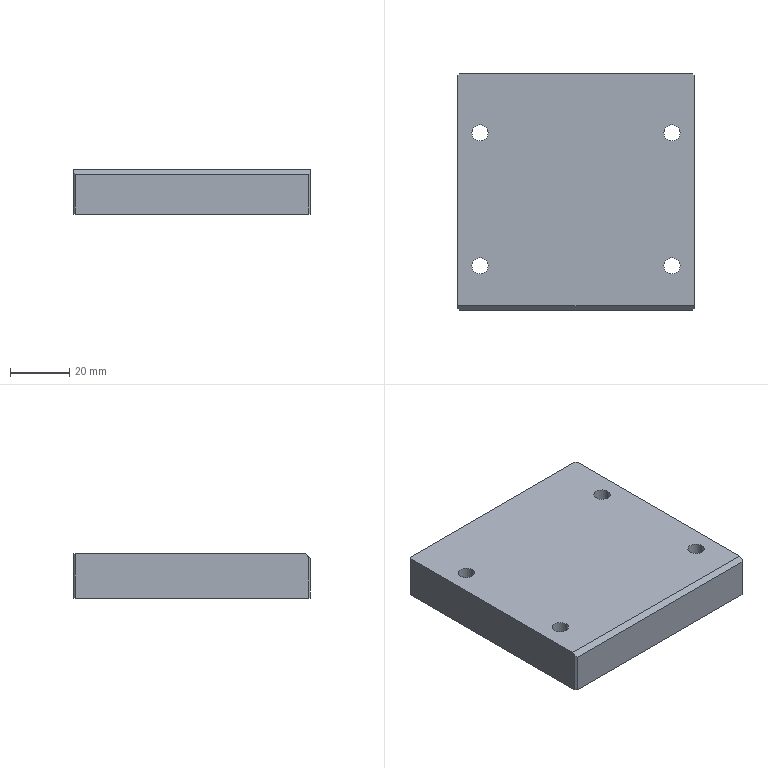Part | SolidWorks | features BaseBody 1 | 1 solid | 43 faces | box 80 x 80 x 15 mm | volume 92315 mm3 | cylinder 22 | plane 15 | cone 6 | commonest cylinder face diameters 5.5 x8 10 x8 5 x6
STEP:
#1=CARTESIAN_POINT('',(-27.5,-25.,5.7));
#2=VERTEX_POINT('',#1);
#3=CARTESIAN_POINT('',(-37.5,-25.,5.7));
#4=VERTEX_POINT('',#3);
#5=CARTESIAN_POINT('',(-32.5,-25.,5.7));
#6=DIRECTION('',(0.,0.,-1.));
#7=DIRECTION('',(-1.,0.,0.));
#8=AXIS2_PLACEMENT_3D('',#5,#6,#7);
#9=CIRCLE('',#8,5.);
#10=EDGE_CURVE('',#2,#4,#9,.T.);
#11=ORIENTED_EDGE('',*,*,#10,.F.);
#12=CARTESIAN_POINT('',(-27.5,-25.,0.));
#13=VERTEX_POINT('',#12);
#14=CARTESIAN_POINT('',(-27.5,-25.,0.));
#15=DIRECTION('',(0.,0.,-1.));
#16=VECTOR('',#15,1000.);
#17=LINE('',#14,#16);
#18=EDGE_CURVE('',#2,#13,#17,.T.);
#19=ORIENTED_EDGE('',*,*,#18,.T.);
#20=CARTESIAN_POINT('',(-37.5,-25.,0.));
#21=VERTEX_POINT('',#20);
#22=CARTESIAN_POINT('',(-32.5,-25.,0.));
#23=DIRECTION('',(0.,0.,-1.));
#24=DIRECTION('',(-1.,0.,0.));
#25=AXIS2_PLACEMENT_3D('',#22,#23,#24);
#26=CIRCLE('',#25,5.);
#27=EDGE_CURVE('',#13,#21,#26,.T.);
#28=ORIENTED_EDGE('',*,*,#27,.T.);
#29=CARTESIAN_POINT('',(-37.5,-25.,0.));
#30=DIRECTION('',(0.,0.,-1.));
#31=VECTOR('',#30,1000.);
#32=LINE('',#29,#31);
#33=EDGE_CURVE('',#4,#21,#32,.T.);
#34=ORIENTED_EDGE('',*,*,#33,.F.);
#35=EDGE_LOOP('',(#11,#19,#28,#34));
#36=FACE_OUTER_BOUND('',#35,.T.);
#37=CARTESIAN_POINT('',(-32.5,-25.,0.));
#38=DIRECTION('',(0.,0.,-1.));
#39=DIRECTION('',(-1.,0.,0.));
#40=AXIS2_PLACEMENT_3D('',#37,#38,#39);
#41=CYLINDRICAL_SURFACE('',#40,5.);
#42=ADVANCED_FACE('',(#36),#41,.F.);
#43=CARTESIAN_POINT('',(-29.75,-25.,15.));
#44=VERTEX_POINT('',#43);
#45=CARTESIAN_POINT('',(-35.25,-25.,15.));
#46=VERTEX_POINT('',#45);
#47=CARTESIAN_POINT('',(-32.5,-25.,15.));
#48=DIRECTION('',(0.,0.,-1.));
#49=DIRECTION('',(-1.,0.,0.));
#50=AXIS2_PLACEMENT_3D('',#47,#48,#49);
#51=CIRCLE('',#50,2.75);
#52=EDGE_CURVE('',#44,#46,#51,.T.);
#53=ORIENTED_EDGE('',*,*,#52,.F.);
#54=CARTESIAN_POINT('',(-29.75,-25.,5.7));
#55=VERTEX_POINT('',#54);
#56=CARTESIAN_POINT('',(-29.75,-25.,0.));
#57=DIRECTION('',(0.,0.,-1.));
#58=VECTOR('',#57,1000.);
#59=LINE('',#56,#58);
#60=EDGE_CURVE('',#44,#55,#59,.T.);
#61=ORIENTED_EDGE('',*,*,#60,.T.);
#62=CARTESIAN_POINT('',(-35.25,-25.,5.7));
#63=VERTEX_POINT('',#62);
#64=CARTESIAN_POINT('',(-32.5,-25.,5.7));
#65=DIRECTION('',(0.,0.,-1.));
#66=DIRECTION('',(-1.,0.,0.));
#67=AXIS2_PLACEMENT_3D('',#64,#65,#66);
#68=CIRCLE('',#67,2.75);
#69=EDGE_CURVE('',#55,#63,#68,.T.);
#70=ORIENTED_EDGE('',*,*,#69,.T.);
#71=CARTESIAN_POINT('',(-35.25,-25.,0.));
#72=DIRECTION('',(0.,0.,-1.));
#73=VECTOR('',#72,1000.);
#74=LINE('',#71,#73);
#75=EDGE_CURVE('',#46,#63,#74,.T.);
#76=ORIENTED_EDGE('',*,*,#75,.F.);
#77=EDGE_LOOP('',(#53,#61,#70,#76));
#78=FACE_OUTER_BOUND('',#77,.T.);
#79=CARTESIAN_POINT('',(-32.5,-25.,0.));
#80=DIRECTION('',(0.,0.,-1.));
#81=DIRECTION('',(-1.,0.,0.));
#82=AXIS2_PLACEMENT_3D('',#79,#80,#81);
#83=CYLINDRICAL_SURFACE('',#82,2.75);
#84=ADVANCED_FACE('',(#78),#83,.F.);
#85=CARTESIAN_POINT('',(-27.5,20.,5.7));
#86=VERTEX_POINT('',#85);
#87=CARTESIAN_POINT('',(-37.5,20.,5.7));
#88=VERTEX_POINT('',#87);
#89=CARTESIAN_POINT('',(-32.5,20.,5.7));
#90=DIRECTION('',(0.,0.,-1.));
#91=DIRECTION('',(-1.,0.,0.));
#92=AXIS2_PLACEMENT_3D('',#89,#90,#91);
#93=CIRCLE('',#92,5.);
#94=EDGE_CURVE('',#86,#88,#93,.T.);
#95=ORIENTED_EDGE('',*,*,#94,.F.);
#96=CARTESIAN_POINT('',(-27.5,20.,0.));
#97=VERTEX_POINT('',#96);
#98=CARTESIAN_POINT('',(-27.5,20.,0.));
#99=DIRECTION('',(0.,0.,-1.));
#100=VECTOR('',#99,1000.);
#101=LINE('',#98,#100);
#102=EDGE_CURVE('',#86,#97,#101,.T.);
#103=ORIENTED_EDGE('',*,*,#102,.T.);
#104=CARTESIAN_POINT('',(-37.5,20.,0.));
#105=VERTEX_POINT('',#104);
#106=CARTESIAN_POINT('',(-32.5,20.,0.));
#107=DIRECTION('',(0.,0.,-1.));
#108=DIRECTION('',(-1.,0.,0.));
#109=AXIS2_PLACEMENT_3D('',#106,#107,#108);
#110=CIRCLE('',#109,5.);
#111=EDGE_CURVE('',#97,#105,#110,.T.);
#112=ORIENTED_EDGE('',*,*,#111,.T.);
#113=CARTESIAN_POINT('',(-37.5,20.,0.));
#114=DIRECTION('',(0.,0.,-1.));
#115=VECTOR('',#114,1000.);
#116=LINE('',#113,#115);
#117=EDGE_CURVE('',#88,#105,#116,.T.);
#118=ORIENTED_EDGE('',*,*,#117,.F.);
#119=EDGE_LOOP('',(#95,#103,#112,#118));
#120=FACE_OUTER_BOUND('',#119,.T.);
#121=CARTESIAN_POINT('',(-32.5,20.,0.));
#122=DIRECTION('',(0.,0.,-1.));
#123=DIRECTION('',(-1.,0.,0.));
#124=AXIS2_PLACEMENT_3D('',#121,#122,#123);
#125=CYLINDRICAL_SURFACE('',#124,5.);
#126=ADVANCED_FACE('',(#120),#125,.F.);
#127=CARTESIAN_POINT('',(-29.75,20.,15.));
#128=VERTEX_POINT('',#127);
#129=CARTESIAN_POINT('',(-35.25,20.,15.));
#130=VERTEX_POINT('',#129);
#131=CARTESIAN_POINT('',(-32.5,20.,15.));
#132=DIRECTION('',(0.,0.,-1.));
#133=DIRECTION('',(-1.,0.,0.));
#134=AXIS2_PLACEMENT_3D('',#131,#132,#133);
#135=CIRCLE('',#134,2.75);
#136=EDGE_CURVE('',#128,#130,#135,.T.);
#137=ORIENTED_EDGE('',*,*,#136,.F.);
#138=CARTESIAN_POINT('',(-29.75,20.,5.7));
#139=VERTEX_POINT('',#138);
#140=CARTESIAN_POINT('',(-29.75,20.,0.));
#141=DIRECTION('',(0.,0.,-1.));
#142=VECTOR('',#141,1000.);
#143=LINE('',#140,#142);
#144=EDGE_CURVE('',#128,#139,#143,.T.);
#145=ORIENTED_EDGE('',*,*,#144,.T.);
#146=CARTESIAN_POINT('',(-35.25,20.,5.7));
#147=VERTEX_POINT('',#146);
#148=CARTESIAN_POINT('',(-32.5,20.,5.7));
#149=DIRECTION('',(0.,0.,-1.));
#150=DIRECTION('',(-1.,0.,0.));
#151=AXIS2_PLACEMENT_3D('',#148,#149,#150);
#152=CIRCLE('',#151,2.75);
#153=EDGE_CURVE('',#139,#147,#152,.T.);
#154=ORIENTED_EDGE('',*,*,#153,.T.);
#155=CARTESIAN_POINT('',(-35.25,20.,0.));
#156=DIRECTION('',(0.,0.,-1.));
#157=VECTOR('',#156,1000.);
#158=LINE('',#155,#157);
#159=EDGE_CURVE('',#130,#147,#158,.T.);
#160=ORIENTED_EDGE('',*,*,#159,.F.);
#161=EDGE_LOOP('',(#137,#145,#154,#160));
#162=FACE_OUTER_BOUND('',#161,.T.);
#163=CARTESIAN_POINT('',(-32.5,20.,0.));
#164=DIRECTION('',(0.,0.,-1.));
#165=DIRECTION('',(-1.,0.,0.));
#166=AXIS2_PLACEMENT_3D('',#163,#164,#165);
#167=CYLINDRICAL_SURFACE('',#166,2.75);
#168=ADVANCED_FACE('',(#162),#167,.F.);
#169=CARTESIAN_POINT('',(37.5,20.,5.7));
#170=VERTEX_POINT('',#169);
#171=CARTESIAN_POINT('',(27.5,20.,5.7));
#172=VERTEX_POINT('',#171);
#173=CARTESIAN_POINT('',(32.5,20.,5.7));
#174=DIRECTION('',(0.,0.,-1.));
#175=DIRECTION('',(-1.,0.,0.));
#176=AXIS2_PLACEMENT_3D('',#173,#174,#175);
#177=CIRCLE('',#176,5.);
#178=EDGE_CURVE('',#170,#172,#177,.T.);
#179=ORIENTED_EDGE('',*,*,#178,.F.);
#180=CARTESIAN_POINT('',(37.5,20.,0.));
#181=VERTEX_POINT('',#180);
#182=CARTESIAN_POINT('',(37.5,20.,0.));
#183=DIRECTION('',(0.,0.,-1.));
#184=VECTOR('',#183,1000.);
#185=LINE('',#182,#184);
#186=EDGE_CURVE('',#170,#181,#185,.T.);
#187=ORIENTED_EDGE('',*,*,#186,.T.);
#188=CARTESIAN_POINT('',(27.5,20.,0.));
#189=VERTEX_POINT('',#188);
#190=CARTESIAN_POINT('',(32.5,20.,0.));
#191=DIRECTION('',(0.,0.,-1.));
#192=DIRECTION('',(-1.,0.,0.));
#193=AXIS2_PLACEMENT_3D('',#190,#191,#192);
#194=CIRCLE('',#193,5.);
#195=EDGE_CURVE('',#181,#189,#194,.T.);
#196=ORIENTED_EDGE('',*,*,#195,.T.);
#197=CARTESIAN_POINT('',(27.5,20.,0.));
#198=DIRECTION('',(0.,0.,-1.));
#199=VECTOR('',#198,1000.);
#200=LINE('',#197,#199);
#201=EDGE_CURVE('',#172,#189,#200,.T.);
#202=ORIENTED_EDGE('',*,*,#201,.F.);
#203=EDGE_LOOP('',(#179,#187,#196,#202));
#204=FACE_OUTER_BOUND('',#203,.T.);
#205=CARTESIAN_POINT('',(32.5,20.,0.));
#206=DIRECTION('',(0.,0.,-1.));
#207=DIRECTION('',(-1.,0.,0.));
#208=AXIS2_PLACEMENT_3D('',#205,#206,#207);
#209=CYLINDRICAL_SURFACE('',#208,5.);
#210=ADVANCED_FACE('',(#204),#209,.F.);
#211=CARTESIAN_POINT('',(35.25,20.,15.));
#212=VERTEX_POINT('',#211);
#213=CARTESIAN_POINT('',(29.75,20.,15.));
#214=VERTEX_POINT('',#213);
#215=CARTESIAN_POINT('',(32.5,20.,15.));
#216=DIRECTION('',(0.,0.,-1.));
#217=DIRECTION('',(-1.,0.,0.));
#218=AXIS2_PLACEMENT_3D('',#215,#216,#217);
#219=CIRCLE('',#218,2.75);
#220=EDGE_CURVE('',#212,#214,#219,.T.);
#221=ORIENTED_EDGE('',*,*,#220,.F.);
#222=CARTESIAN_POINT('',(35.25,20.,5.7));
#223=VERTEX_POINT('',#222);
#224=CARTESIAN_POINT('',(35.25,20.,0.));
#225=DIRECTION('',(0.,0.,-1.));
#226=VECTOR('',#225,1000.);
#227=LINE('',#224,#226);
#228=EDGE_CURVE('',#212,#223,#227,.T.);
#229=ORIENTED_EDGE('',*,*,#228,.T.);
#230=CARTESIAN_POINT('',(29.75,20.,5.7));
#231=VERTEX_POINT('',#230);
#232=CARTESIAN_POINT('',(32.5,20.,5.7));
#233=DIRECTION('',(0.,0.,-1.));
#234=DIRECTION('',(-1.,0.,0.));
#235=AXIS2_PLACEMENT_3D('',#232,#233,#234);
#236=CIRCLE('',#235,2.75);
#237=EDGE_CURVE('',#223,#231,#236,.T.);
#238=ORIENTED_EDGE('',*,*,#237,.T.);
#239=CARTESIAN_POINT('',(29.75,20.,0.));
#240=DIRECTION('',(0.,0.,-1.));
#241=VECTOR('',#240,1000.);
#242=LINE('',#239,#241);
#243=EDGE_CURVE('',#214,#231,#242,.T.);
#244=ORIENTED_EDGE('',*,*,#243,.F.);
#245=EDGE_LOOP('',(#221,#229,#238,#244));
#246=FACE_OUTER_BOUND('',#245,.T.);
#247=CARTESIAN_POINT('',(32.5,20.,0.));
#248=DIRECTION('',(0.,0.,-1.));
#249=DIRECTION('',(-1.,0.,0.));
#250=AXIS2_PLACEMENT_3D('',#247,#248,#249);
#251=CYLINDRICAL_SURFACE('',#250,2.75);
#252=ADVANCED_FACE('',(#246),#251,.F.);
#253=CARTESIAN_POINT('',(37.5,-25.,5.7));
#254=VERTEX_POINT('',#253);
#255=CARTESIAN_POINT('',(27.5,-25.,5.7));
#256=VERTEX_POINT('',#255);
#257=CARTESIAN_POINT('',(32.5,-25.,5.7));
#258=DIRECTION('',(0.,0.,-1.));
#259=DIRECTION('',(-1.,0.,0.));
#260=AXIS2_PLACEMENT_3D('',#257,#258,#259);
#261=CIRCLE('',#260,5.);
#262=EDGE_CURVE('',#254,#256,#261,.T.);
#263=ORIENTED_EDGE('',*,*,#262,.F.);
#264=CARTESIAN_POINT('',(37.5,-25.,0.));
#265=VERTEX_POINT('',#264);
#266=CARTESIAN_POINT('',(37.5,-25.,0.));
#267=DIRECTION('',(0.,0.,-1.));
#268=VECTOR('',#267,1000.);
#269=LINE('',#266,#268);
#270=EDGE_CURVE('',#254,#265,#269,.T.);
#271=ORIENTED_EDGE('',*,*,#270,.T.);
#272=CARTESIAN_POINT('',(27.5,-25.,0.));
#273=VERTEX_POINT('',#272);
#274=CARTESIAN_POINT('',(32.5,-25.,0.));
#275=DIRECTION('',(0.,0.,-1.));
#276=DIRECTION('',(-1.,0.,0.));
#277=AXIS2_PLACEMENT_3D('',#274,#275,#276);
#278=CIRCLE('',#277,5.);
#279=EDGE_CURVE('',#265,#273,#278,.T.);
#280=ORIENTED_EDGE('',*,*,#279,.T.);
#281=CARTESIAN_POINT('',(27.5,-25.,0.));
#282=DIRECTION('',(0.,0.,-1.));
#283=VECTOR('',#282,1000.);
#284=LINE('',#281,#283);
#285=EDGE_CURVE('',#256,#273,#284,.T.);
#286=ORIENTED_EDGE('',*,*,#285,.F.);
#287=EDGE_LOOP('',(#263,#271,#280,#286));
#288=FACE_OUTER_BOUND('',#287,.T.);
#289=CARTESIAN_POINT('',(32.5,-25.,0.));
#290=DIRECTION('',(0.,0.,-1.));
#291=DIRECTION('',(-1.,0.,0.));
#292=AXIS2_PLACEMENT_3D('',#289,#290,#291);
#293=CYLINDRICAL_SURFACE('',#292,5.);
#294=ADVANCED_FACE('',(#288),#293,.F.);
#295=CARTESIAN_POINT('',(35.25,-25.,15.));
#296=VERTEX_POINT('',#295);
#297=CARTESIAN_POINT('',(29.75,-25.,15.));
#298=VERTEX_POINT('',#297);
#299=CARTESIAN_POINT('',(32.5,-25.,15.));
#300=DIRECTION('',(0.,0.,-1.));
#301=DIRECTION('',(-1.,0.,0.));
#302=AXIS2_PLACEMENT_3D('',#299,#300,#301);
#303=CIRCLE('',#302,2.75);
#304=EDGE_CURVE('',#296,#298,#303,.T.);
#305=ORIENTED_EDGE('',*,*,#304,.F.);
#306=CARTESIAN_POINT('',(35.25,-25.,5.7));
#307=VERTEX_POINT('',#306);
#308=CARTESIAN_POINT('',(35.25,-25.,0.));
#309=DIRECTION('',(0.,0.,-1.));
#310=VECTOR('',#309,1000.);
#311=LINE('',#308,#310);
#312=EDGE_CURVE('',#296,#307,#311,.T.);
#313=ORIENTED_EDGE('',*,*,#312,.T.);
#314=CARTESIAN_POINT('',(29.75,-25.,5.7));
#315=VERTEX_POINT('',#314);
#316=CARTESIAN_POINT('',(32.5,-25.,5.7));
#317=DIRECTION('',(0.,0.,-1.));
#318=DIRECTION('',(-1.,0.,0.));
#319=AXIS2_PLACEMENT_3D('',#316,#317,#318);
#320=CIRCLE('',#319,2.75);
#321=EDGE_CURVE('',#307,#315,#320,.T.);
#322=ORIENTED_EDGE('',*,*,#321,.T.);
#323=CARTESIAN_POINT('',(29.75,-25.,0.));
#324=DIRECTION('',(0.,0.,-1.));
#325=VECTOR('',#324,1000.);
#326=LINE('',#323,#325);
#327=EDGE_CURVE('',#298,#315,#326,.T.);
#328=ORIENTED_EDGE('',*,*,#327,.F.);
#329=EDGE_LOOP('',(#305,#313,#322,#328));
#330=FACE_OUTER_BOUND('',#329,.T.);
#331=CARTESIAN_POINT('',(32.5,-25.,0.));
#332=DIRECTION('',(0.,0.,-1.));
#333=DIRECTION('',(-1.,0.,0.));
#334=AXIS2_PLACEMENT_3D('',#331,#332,#333);
#335=CYLINDRICAL_SURFACE('',#334,2.75);
#336=ADVANCED_FACE('',(#330),#335,.F.);
#337=CARTESIAN_POINT('',(-27.5,25.,5.));
#338=VERTEX_POINT('',#337);
#339=CARTESIAN_POINT('',(-27.5,25.,10.));
#340=VERTEX_POINT('',#339);
#341=CARTESIAN_POINT('',(-27.5,25.,7.5));
#342=DIRECTION('',(0.,1.,0.));
#343=DIRECTION('',(0.,0.,1.));
#344=AXIS2_PLACEMENT_3D('',#341,#342,#343);
#345=CIRCLE('',#344,2.5);
#346=EDGE_CURVE('',#338,#340,#345,.T.);
#347=ORIENTED_EDGE('',*,*,#346,.F.);
#348=CARTESIAN_POINT('',(-27.5,40.,5.));
#349=VERTEX_POINT('',#348);
#350=CARTESIAN_POINT('',(-27.5,40.,5.));
#351=DIRECTION('',(0.,1.,0.));
#352=VECTOR('',#351,1000.);
#353=LINE('',#350,#352);
#354=EDGE_CURVE('',#338,#349,#353,.T.);
#355=ORIENTED_EDGE('',*,*,#354,.T.);
#356=CARTESIAN_POINT('',(-27.5,40.,10.));
#357=VERTEX_POINT('',#356);
#358=CARTESIAN_POINT('',(-27.5,40.,7.5));
#359=DIRECTION('',(0.,1.,0.));
#360=DIRECTION('',(0.,0.,1.));
#361=AXIS2_PLACEMENT_3D('',#358,#359,#360);
#362=CIRCLE('',#361,2.5);
#363=EDGE_CURVE('',#349,#357,#362,.T.);
#364=ORIENTED_EDGE('',*,*,#363,.T.);
#365=CARTESIAN_POINT('',(-27.5,40.,10.));
#366=DIRECTION('',(0.,1.,0.));
#367=VECTOR('',#366,1000.);
#368=LINE('',#365,#367);
#369=EDGE_CURVE('',#340,#357,#368,.T.);
#370=ORIENTED_EDGE('',*,*,#369,.F.);
#371=EDGE_LOOP('',(#347,#355,#364,#370));
#372=FACE_OUTER_BOUND('',#371,.T.);
#373=CARTESIAN_POINT('',(-27.5,40.,7.5));
#374=DIRECTION('',(0.,1.,0.));
#375=DIRECTION('',(0.,0.,1.));
#376=AXIS2_PLACEMENT_3D('',#373,#374,#375);
#377=CYLINDRICAL_SURFACE('',#376,2.5);
#378=ADVANCED_FACE('',(#372),#377,.F.);
#379=CARTESIAN_POINT('',(-27.5,23.498,7.5));
#380=VERTEX_POINT('',#379);
#381=CARTESIAN_POINT('',(-27.5,25.,10.));
#382=DIRECTION('',(0.,0.515,0.8572));
#383=VECTOR('',#382,1000.);
#384=LINE('',#381,#383);
#385=EDGE_CURVE('',#380,#340,#384,.T.);
#386=ORIENTED_EDGE('',*,*,#385,.F.);
#387=CARTESIAN_POINT('',(-27.5,25.,5.));
#388=DIRECTION('',(0.,0.515,-0.8572));
#389=VECTOR('',#388,1000.);
#390=LINE('',#387,#389);
#391=EDGE_CURVE('',#380,#338,#390,.T.);
#392=ORIENTED_EDGE('',*,*,#391,.T.);
#393=ORIENTED_EDGE('',*,*,#346,.T.);
#394=EDGE_LOOP('',(#386,#392,#393));
#395=FACE_OUTER_BOUND('',#394,.T.);
#396=CARTESIAN_POINT('',(-27.5,25.,7.5));
#397=DIRECTION('',(0.,1.,0.));
#398=DIRECTION('',(0.,0.,1.));
#399=AXIS2_PLACEMENT_3D('',#396,#397,#398);
#400=CONICAL_SURFACE('',#399,2.5,1.03);
#401=ADVANCED_FACE('',(#395),#400,.F.);
#402=CARTESIAN_POINT('',(0.,25.,5.));
#403=VERTEX_POINT('',#402);
#404=CARTESIAN_POINT('',(0.,25.,10.));
#405=VERTEX_POINT('',#404);
#406=CARTESIAN_POINT('',(0.,25.,7.5));
#407=DIRECTION('',(0.,1.,0.));
#408=DIRECTION('',(0.,0.,1.));
#409=AXIS2_PLACEMENT_3D('',#406,#407,#408);
#410=CIRCLE('',#409,2.5);
#411=EDGE_CURVE('',#403,#405,#410,.T.);
#412=ORIENTED_EDGE('',*,*,#411,.F.);
#413=CARTESIAN_POINT('',(0.,40.,5.));
#414=VERTEX_POINT('',#413);
#415=CARTESIAN_POINT('',(0.,40.,5.));
#416=DIRECTION('',(0.,1.,0.));
#417=VECTOR('',#416,1000.);
#418=LINE('',#415,#417);
#419=EDGE_CURVE('',#403,#414,#418,.T.);
#420=ORIENTED_EDGE('',*,*,#419,.T.);
#421=CARTESIAN_POINT('',(0.,40.,10.));
#422=VERTEX_POINT('',#421);
#423=CARTESIAN_POINT('',(0.,40.,7.5));
#424=DIRECTION('',(0.,1.,0.));
#425=DIRECTION('',(0.,0.,1.));
#426=AXIS2_PLACEMENT_3D('',#423,#424,#425);
#427=CIRCLE('',#426,2.5);
#428=EDGE_CURVE('',#414,#422,#427,.T.);
#429=ORIENTED_EDGE('',*,*,#428,.T.);
#430=CARTESIAN_POINT('',(0.,40.,10.));
#431=DIRECTION('',(0.,1.,0.));
#432=VECTOR('',#431,1000.);
#433=LINE('',#430,#432);
#434=EDGE_CURVE('',#405,#422,#433,.T.);
#435=ORIENTED_EDGE('',*,*,#434,.F.);
#436=EDGE_LOOP('',(#412,#420,#429,#435));
#437=FACE_OUTER_BOUND('',#436,.T.);
#438=CARTESIAN_POINT('',(0.,40.,7.5));
#439=DIRECTION('',(0.,1.,0.));
#440=DIRECTION('',(0.,0.,1.));
#441=AXIS2_PLACEMENT_3D('',#438,#439,#440);
#442=CYLINDRICAL_SURFACE('',#441,2.5);
#443=ADVANCED_FACE('',(#437),#442,.F.);
#444=CARTESIAN_POINT('',(0.,23.498,7.5));
#445=VERTEX_POINT('',#444);
#446=CARTESIAN_POINT('',(0.,25.,10.));
#447=DIRECTION('',(0.,0.515,0.8572));
#448=VECTOR('',#447,1000.);
#449=LINE('',#446,#448);
#450=EDGE_CURVE('',#445,#405,#449,.T.);
#451=ORIENTED_EDGE('',*,*,#450,.F.);
#452=CARTESIAN_POINT('',(0.,25.,5.));
#453=DIRECTION('',(0.,0.515,-0.8572));
#454=VECTOR('',#453,1000.);
#455=LINE('',#452,#454);
#456=EDGE_CURVE('',#445,#403,#455,.T.);
#457=ORIENTED_EDGE('',*,*,#456,.T.);
#458=ORIENTED_EDGE('',*,*,#411,.T.);
#459=EDGE_LOOP('',(#451,#457,#458));
#460=FACE_OUTER_BOUND('',#459,.T.);
#461=CARTESIAN_POINT('',(0.,25.,7.5));
#462=DIRECTION('',(0.,1.,0.));
#463=DIRECTION('',(0.,0.,1.));
#464=AXIS2_PLACEMENT_3D('',#461,#462,#463);
#465=CONICAL_SURFACE('',#464,2.5,1.03);
#466=ADVANCED_FACE('',(#460),#465,.F.);
#467=CARTESIAN_POINT('',(27.5,25.,5.));
#468=VERTEX_POINT('',#467);
#469=CARTESIAN_POINT('',(27.5,25.,10.));
#470=VERTEX_POINT('',#469);
#471=CARTESIAN_POINT('',(27.5,25.,7.5));
#472=DIRECTION('',(0.,1.,0.));
#473=DIRECTION('',(0.,0.,1.));
#474=AXIS2_PLACEMENT_3D('',#471,#472,#473);
#475=CIRCLE('',#474,2.5);
#476=EDGE_CURVE('',#468,#470,#475,.T.);
#477=ORIENTED_EDGE('',*,*,#476,.F.);
#478=CARTESIAN_POINT('',(27.5,40.,5.));
#479=VERTEX_POINT('',#478);
#480=CARTESIAN_POINT('',(27.5,40.,5.));
#481=DIRECTION('',(0.,1.,0.));
#482=VECTOR('',#481,1000.);
#483=LINE('',#480,#482);
#484=EDGE_CURVE('',#468,#479,#483,.T.);
#485=ORIENTED_EDGE('',*,*,#484,.T.);
#486=CARTESIAN_POINT('',(27.5,40.,10.));
#487=VERTEX_POINT('',#486);
#488=CARTESIAN_POINT('',(27.5,40.,7.5));
#489=DIRECTION('',(0.,1.,0.));
#490=DIRECTION('',(0.,0.,1.));
#491=AXIS2_PLACEMENT_3D('',#488,#489,#490);
#492=CIRCLE('',#491,2.5);
#493=EDGE_CURVE('',#479,#487,#492,.T.);
#494=ORIENTED_EDGE('',*,*,#493,.T.);
#495=CARTESIAN_POINT('',(27.5,40.,10.));
#496=DIRECTION('',(0.,1.,0.));
#497=VECTOR('',#496,1000.);
#498=LINE('',#495,#497);
#499=EDGE_CURVE('',#470,#487,#498,.T.);
#500=ORIENTED_EDGE('',*,*,#499,.F.);
#501=EDGE_LOOP('',(#477,#485,#494,#500));
#502=FACE_OUTER_BOUND('',#501,.T.);
#503=CARTESIAN_POINT('',(27.5,40.,7.5));
#504=DIRECTION('',(0.,1.,0.));
#505=DIRECTION('',(0.,0.,1.));
#506=AXIS2_PLACEMENT_3D('',#503,#504,#505);
#507=CYLINDRICAL_SURFACE('',#506,2.5);
#508=ADVANCED_FACE('',(#502),#507,.F.);
#509=CARTESIAN_POINT('',(27.5,23.498,7.5));
#510=VERTEX_POINT('',#509);
#511=CARTESIAN_POINT('',(27.5,25.,10.));
#512=DIRECTION('',(0.,0.515,0.8572));
#513=VECTOR('',#512,1000.);
#514=LINE('',#511,#513);
#515=EDGE_CURVE('',#510,#470,#514,.T.);
#516=ORIENTED_EDGE('',*,*,#515,.F.);
#517=CARTESIAN_POINT('',(27.5,25.,5.));
#518=DIRECTION('',(0.,0.515,-0.8572));
#519=VECTOR('',#518,1000.);
#520=LINE('',#517,#519);
#521=EDGE_CURVE('',#510,#468,#520,.T.);
#522=ORIENTED_EDGE('',*,*,#521,.T.);
#523=ORIENTED_EDGE('',*,*,#476,.T.);
#524=EDGE_LOOP('',(#516,#522,#523));
#525=FACE_OUTER_BOUND('',#524,.T.);
#526=CARTESIAN_POINT('',(27.5,25.,7.5));
#527=DIRECTION('',(0.,1.,0.));
#528=DIRECTION('',(0.,0.,1.));
#529=AXIS2_PLACEMENT_3D('',#526,#527,#528);
#530=CONICAL_SURFACE('',#529,2.5,1.03);
#531=ADVANCED_FACE('',(#525),#530,.F.);
#532=CARTESIAN_POINT('',(-39.5,-40.,13.5));
#533=VERTEX_POINT('',#532);
#534=CARTESIAN_POINT('',(-40.,-39.5,14.));
#535=VERTEX_POINT('',#534);
#536=CARTESIAN_POINT('',(-40.,-39.5,14.));
#537=DIRECTION('',(-0.5774,0.5774,0.5774));
#538=VECTOR('',#537,1000.);
#539=LINE('',#536,#538);
#540=EDGE_CURVE('',#533,#535,#539,.T.);
#541=ORIENTED_EDGE('',*,*,#540,.F.);
#542=CARTESIAN_POINT('',(39.5,-40.,13.5));
#543=VERTEX_POINT('',#542);
#544=CARTESIAN_POINT('',(-40.,-40.,13.5));
#545=DIRECTION('',(-1.,0.,0.));
#546=VECTOR('',#545,1000.);
#547=LINE('',#544,#546);
#548=EDGE_CURVE('',#543,#533,#547,.T.);
#549=ORIENTED_EDGE('',*,*,#548,.F.);
#550=CARTESIAN_POINT('',(40.,-39.5,14.));
#551=VERTEX_POINT('',#550);
#552=CARTESIAN_POINT('',(40.333,-39.167,14.333));
#553=DIRECTION('',(-0.5774,-0.5774,-0.5774));
#554=VECTOR('',#553,1000.);
#555=LINE('',#552,#554);
#556=EDGE_CURVE('',#551,#543,#555,.T.);
#557=ORIENTED_EDGE('',*,*,#556,.F.);
#558=CARTESIAN_POINT('',(40.,-38.5,15.));
#559=VERTEX_POINT('',#558);
#560=CARTESIAN_POINT('',(40.,-38.5,15.));
#561=DIRECTION('',(0.,-0.7071,-0.7071));
#562=VECTOR('',#561,1000.);
#563=LINE('',#560,#562);
#564=EDGE_CURVE('',#559,#551,#563,.T.);
#565=ORIENTED_EDGE('',*,*,#564,.F.);
#566=CARTESIAN_POINT('',(-40.,-38.5,15.));
#567=VERTEX_POINT('',#566);
#568=CARTESIAN_POINT('',(0.,-38.5,15.));
#569=DIRECTION('',(1.,0.,0.));
#570=VECTOR('',#569,1000.);
#571=LINE('',#568,#570);
#572=EDGE_CURVE('',#567,#559,#571,.T.);
#573=ORIENTED_EDGE('',*,*,#572,.F.);
#574=CARTESIAN_POINT('',(-40.,-38.5,15.));
#575=DIRECTION('',(0.,0.7071,0.7071));
#576=VECTOR('',#575,1000.);
#577=LINE('',#574,#576);
#578=EDGE_CURVE('',#535,#567,#577,.T.);
#579=ORIENTED_EDGE('',*,*,#578,.F.);
#580=EDGE_LOOP('',(#541,#549,#557,#565,#573,#579));
#581=FACE_OUTER_BOUND('',#580,.T.);
#582=CARTESIAN_POINT('',(0.,-38.5,15.));
#583=DIRECTION('',(0.,0.7071,-0.7071));
#584=DIRECTION('',(-1.,0.,0.));
#585=AXIS2_PLACEMENT_3D('',#582,#583,#584);
#586=PLANE('',#585);
#587=ADVANCED_FACE('',(#581),#586,.F.);
#588=CARTESIAN_POINT('',(40.,-39.5,0.));
#589=VERTEX_POINT('',#588);
#590=CARTESIAN_POINT('',(40.,-39.5,15.));
#591=DIRECTION('',(0.,0.,-1.));
#592=VECTOR('',#591,1000.);
#593=LINE('',#590,#592);
#594=EDGE_CURVE('',#551,#589,#593,.T.);
#595=ORIENTED_EDGE('',*,*,#594,.F.);
#596=ORIENTED_EDGE('',*,*,#556,.T.);
#597=CARTESIAN_POINT('',(39.5,-40.,0.));
#598=VERTEX_POINT('',#597);
#599=CARTESIAN_POINT('',(39.5,-40.,15.));
#600=DIRECTION('',(0.,0.,1.));
#601=VECTOR('',#600,1000.);
#602=LINE('',#599,#601);
#603=EDGE_CURVE('',#598,#543,#602,.T.);
#604=ORIENTED_EDGE('',*,*,#603,.F.);
#605=CARTESIAN_POINT('',(39.75,-39.75,0.));
#606=DIRECTION('',(-0.7071,-0.7071,0.));
#607=VECTOR('',#606,1000.);
#608=LINE('',#605,#607);
#609=EDGE_CURVE('',#589,#598,#608,.T.);
#610=ORIENTED_EDGE('',*,*,#609,.F.);
#611=EDGE_LOOP('',(#595,#596,#604,#610));
#612=FACE_OUTER_BOUND('',#611,.T.);
#613=CARTESIAN_POINT('',(40.,-39.5,15.));
#614=DIRECTION('',(-0.7071,0.7071,0.));
#615=DIRECTION('',(0.,0.,1.));
#616=AXIS2_PLACEMENT_3D('',#613,#614,#615);
#617=PLANE('',#616);
#618=ADVANCED_FACE('',(#612),#617,.F.);
#619=CARTESIAN_POINT('',(-39.5,-40.,0.));
#620=VERTEX_POINT('',#619);
#621=CARTESIAN_POINT('',(-39.5,-40.,15.));
#622=DIRECTION('',(0.,0.,-1.));
#623=VECTOR('',#622,1000.);
#624=LINE('',#621,#623);
#625=EDGE_CURVE('',#533,#620,#624,.T.);
#626=ORIENTED_EDGE('',*,*,#625,.F.);
#627=ORIENTED_EDGE('',*,*,#540,.T.);
#628=CARTESIAN_POINT('',(-40.,-39.5,0.));
#629=VERTEX_POINT('',#628);
#630=CARTESIAN_POINT('',(-40.,-39.5,15.));
#631=DIRECTION('',(0.,0.,1.));
#632=VECTOR('',#631,1000.);
#633=LINE('',#630,#632);
#634=EDGE_CURVE('',#629,#535,#633,.T.);
#635=ORIENTED_EDGE('',*,*,#634,.F.);
#636=CARTESIAN_POINT('',(-39.75,-39.75,0.));
#637=DIRECTION('',(-0.7071,0.7071,0.));
#638=VECTOR('',#637,1000.);
#639=LINE('',#636,#638);
#640=EDGE_CURVE('',#620,#629,#639,.T.);
#641=ORIENTED_EDGE('',*,*,#640,.F.);
#642=EDGE_LOOP('',(#626,#627,#635,#641));
#643=FACE_OUTER_BOUND('',#642,.T.);
#644=CARTESIAN_POINT('',(-39.5,-40.,15.));
#645=DIRECTION('',(0.7071,0.7071,0.));
#646=DIRECTION('',(0.,0.,-1.));
#647=AXIS2_PLACEMENT_3D('',#644,#645,#646);
#648=PLANE('',#647);
#649=ADVANCED_FACE('',(#643),#648,.F.);
#650=CARTESIAN_POINT('',(40.,39.5,15.));
#651=VERTEX_POINT('',#650);
#652=CARTESIAN_POINT('',(39.5,40.,15.));
#653=VERTEX_POINT('',#652);
#654=CARTESIAN_POINT('',(39.5,40.,15.));
#655=DIRECTION('',(-0.7071,0.7071,0.));
#656=VECTOR('',#655,1000.);
#657=LINE('',#654,#656);
#658=EDGE_CURVE('',#651,#653,#657,.T.);
#659=ORIENTED_EDGE('',*,*,#658,.F.);
#660=CARTESIAN_POINT('',(40.,39.5,0.));
#661=VERTEX_POINT('',#660);
#662=CARTESIAN_POINT('',(40.,39.5,15.));
#663=DIRECTION('',(0.,0.,1.));
#664=VECTOR('',#663,1000.);
#665=LINE('',#662,#664);
#666=EDGE_CURVE('',#661,#651,#665,.T.);
#667=ORIENTED_EDGE('',*,*,#666,.F.);
#668=CARTESIAN_POINT('',(39.5,40.,0.));
#669=VERTEX_POINT('',#668);
#670=CARTESIAN_POINT('',(39.75,39.75,0.));
#671=DIRECTION('',(0.7071,-0.7071,0.));
#672=VECTOR('',#671,1000.);
#673=LINE('',#670,#672);
#674=EDGE_CURVE('',#669,#661,#673,.T.);
#675=ORIENTED_EDGE('',*,*,#674,.F.);
#676=CARTESIAN_POINT('',(39.5,40.,15.));
#677=DIRECTION('',(0.,0.,-1.));
#678=VECTOR('',#677,1000.);
#679=LINE('',#676,#678);
#680=EDGE_CURVE('',#653,#669,#679,.T.);
#681=ORIENTED_EDGE('',*,*,#680,.F.);
#682=EDGE_LOOP('',(#659,#667,#675,#681));
#683=FACE_OUTER_BOUND('',#682,.T.);
#684=CARTESIAN_POINT('',(39.5,40.,15.));
#685=DIRECTION('',(-0.7071,-0.7071,0.));
#686=DIRECTION('',(-0.7071,0.7071,0.));
#687=AXIS2_PLACEMENT_3D('',#684,#685,#686);
#688=PLANE('',#687);
#689=ADVANCED_FACE('',(#683),#688,.F.);
#690=CARTESIAN_POINT('',(-39.5,40.,15.));
#691=VERTEX_POINT('',#690);
#692=CARTESIAN_POINT('',(-40.,39.5,15.));
#693=VERTEX_POINT('',#692);
#694=CARTESIAN_POINT('',(-40.,39.5,15.));
#695=DIRECTION('',(-0.7071,-0.7071,0.));
#696=VECTOR('',#695,1000.);
#697=LINE('',#694,#696);
#698=EDGE_CURVE('',#691,#693,#697,.T.);
#699=ORIENTED_EDGE('',*,*,#698,.F.);
#700=CARTESIAN_POINT('',(-39.5,40.,0.));
#701=VERTEX_POINT('',#700);
#702=CARTESIAN_POINT('',(-39.5,40.,15.));
#703=DIRECTION('',(0.,0.,1.));
#704=VECTOR('',#703,1000.);
#705=LINE('',#702,#704);
#706=EDGE_CURVE('',#701,#691,#705,.T.);
#707=ORIENTED_EDGE('',*,*,#706,.F.);
#708=CARTESIAN_POINT('',(-40.,39.5,0.));
#709=VERTEX_POINT('',#708);
#710=CARTESIAN_POINT('',(-39.75,39.75,0.));
#711=DIRECTION('',(0.7071,0.7071,0.));
#712=VECTOR('',#711,1000.);
#713=LINE('',#710,#712);
#714=EDGE_CURVE('',#709,#701,#713,.T.);
#715=ORIENTED_EDGE('',*,*,#714,.F.);
#716=CARTESIAN_POINT('',(-40.,39.5,15.));
#717=DIRECTION('',(0.,0.,-1.));
#718=VECTOR('',#717,1000.);
#719=LINE('',#716,#718);
#720=EDGE_CURVE('',#693,#709,#719,.T.);
#721=ORIENTED_EDGE('',*,*,#720,.F.);
#722=EDGE_LOOP('',(#699,#707,#715,#721));
#723=FACE_OUTER_BOUND('',#722,.T.);
#724=CARTESIAN_POINT('',(-40.,39.5,15.));
#725=DIRECTION('',(0.7071,-0.7071,0.));
#726=DIRECTION('',(0.,0.,-1.));
#727=AXIS2_PLACEMENT_3D('',#724,#725,#726);
#728=PLANE('',#727);
#729=ADVANCED_FACE('',(#723),#728,.F.);
#730=CARTESIAN_POINT('',(-32.5,-25.,5.7));
#731=DIRECTION('',(0.,0.,-1.));
#732=DIRECTION('',(-1.,0.,0.));
#733=AXIS2_PLACEMENT_3D('',#730,#731,#732);
#734=CIRCLE('',#733,2.75);
#735=EDGE_CURVE('',#63,#55,#734,.T.);
#736=ORIENTED_EDGE('',*,*,#735,.F.);
#737=ORIENTED_EDGE('',*,*,#69,.F.);
#738=EDGE_LOOP('',(#736,#737));
#739=FACE_BOUND('',#738,.T.);
#740=CARTESIAN_POINT('',(-32.5,-25.,5.7));
#741=DIRECTION('',(0.,0.,-1.));
#742=DIRECTION('',(-1.,0.,0.));
#743=AXIS2_PLACEMENT_3D('',#740,#741,#742);
#744=CIRCLE('',#743,5.);
#745=EDGE_CURVE('',#4,#2,#744,.T.);
#746=ORIENTED_EDGE('',*,*,#745,.T.);
#747=ORIENTED_EDGE('',*,*,#10,.T.);
#748=EDGE_LOOP('',(#746,#747));
#749=FACE_OUTER_BOUND('',#748,.T.);
#750=CARTESIAN_POINT('',(-29.75,-25.,5.7));
#751=DIRECTION('',(0.,0.,1.));
#752=DIRECTION('',(1.,0.,0.));
#753=AXIS2_PLACEMENT_3D('',#750,#751,#752);
#754=PLANE('',#753);
#755=ADVANCED_FACE('',(#739,#749),#754,.F.);
#756=CARTESIAN_POINT('',(-32.5,20.,5.7));
#757=DIRECTION('',(0.,0.,-1.));
#758=DIRECTION('',(-1.,0.,0.));
#759=AXIS2_PLACEMENT_3D('',#756,#757,#758);
#760=CIRCLE('',#759,2.75);
#761=EDGE_CURVE('',#147,#139,#760,.T.);
#762=ORIENTED_EDGE('',*,*,#761,.F.);
#763=ORIENTED_EDGE('',*,*,#153,.F.);
#764=EDGE_LOOP('',(#762,#763));
#765=FACE_BOUND('',#764,.T.);
#766=CARTESIAN_POINT('',(-32.5,20.,5.7));
#767=DIRECTION('',(0.,0.,-1.));
#768=DIRECTION('',(-1.,0.,0.));
#769=AXIS2_PLACEMENT_3D('',#766,#767,#768);
#770=CIRCLE('',#769,5.);
#771=EDGE_CURVE('',#88,#86,#770,.T.);
#772=ORIENTED_EDGE('',*,*,#771,.T.);
#773=ORIENTED_EDGE('',*,*,#94,.T.);
#774=EDGE_LOOP('',(#772,#773));
#775=FACE_OUTER_BOUND('',#774,.T.);
#776=CARTESIAN_POINT('',(-29.75,20.,5.7));
#777=DIRECTION('',(0.,0.,1.));
#778=DIRECTION('',(1.,0.,0.));
#779=AXIS2_PLACEMENT_3D('',#776,#777,#778);
#780=PLANE('',#779);
#781=ADVANCED_FACE('',(#765,#775),#780,.F.);
#782=CARTESIAN_POINT('',(32.5,20.,5.7));
#783=DIRECTION('',(0.,0.,-1.));
#784=DIRECTION('',(-1.,0.,0.));
#785=AXIS2_PLACEMENT_3D('',#782,#783,#784);
#786=CIRCLE('',#785,2.75);
#787=EDGE_CURVE('',#231,#223,#786,.T.);
#788=ORIENTED_EDGE('',*,*,#787,.F.);
#789=ORIENTED_EDGE('',*,*,#237,.F.);
#790=EDGE_LOOP('',(#788,#789));
#791=FACE_BOUND('',#790,.T.);
#792=CARTESIAN_POINT('',(32.5,20.,5.7));
#793=DIRECTION('',(0.,0.,-1.));
#794=DIRECTION('',(-1.,0.,0.));
#795=AXIS2_PLACEMENT_3D('',#792,#793,#794);
#796=CIRCLE('',#795,5.);
#797=EDGE_CURVE('',#172,#170,#796,.T.);
#798=ORIENTED_EDGE('',*,*,#797,.T.);
#799=ORIENTED_EDGE('',*,*,#178,.T.);
#800=EDGE_LOOP('',(#798,#799));
#801=FACE_OUTER_BOUND('',#800,.T.);
#802=CARTESIAN_POINT('',(35.25,20.,5.7));
#803=DIRECTION('',(0.,0.,1.));
#804=DIRECTION('',(1.,0.,0.));
#805=AXIS2_PLACEMENT_3D('',#802,#803,#804);
#806=PLANE('',#805);
#807=ADVANCED_FACE('',(#791,#801),#806,.F.);
#808=CARTESIAN_POINT('',(32.5,-25.,5.7));
#809=DIRECTION('',(0.,0.,-1.));
#810=DIRECTION('',(-1.,0.,0.));
#811=AXIS2_PLACEMENT_3D('',#808,#809,#810);
#812=CIRCLE('',#811,2.75);
#813=EDGE_CURVE('',#315,#307,#812,.T.);
#814=ORIENTED_EDGE('',*,*,#813,.F.);
#815=ORIENTED_EDGE('',*,*,#321,.F.);
#816=EDGE_LOOP('',(#814,#815));
#817=FACE_BOUND('',#816,.T.);
#818=CARTESIAN_POINT('',(32.5,-25.,5.7));
#819=DIRECTION('',(0.,0.,-1.));
#820=DIRECTION('',(-1.,0.,0.));
#821=AXIS2_PLACEMENT_3D('',#818,#819,#820);
#822=CIRCLE('',#821,5.);
#823=EDGE_CURVE('',#256,#254,#822,.T.);
#824=ORIENTED_EDGE('',*,*,#823,.T.);
#825=ORIENTED_EDGE('',*,*,#262,.T.);
#826=EDGE_LOOP('',(#824,#825));
#827=FACE_OUTER_BOUND('',#826,.T.);
#828=CARTESIAN_POINT('',(35.25,-25.,5.7));
#829=DIRECTION('',(0.,0.,1.));
#830=DIRECTION('',(1.,0.,0.));
#831=AXIS2_PLACEMENT_3D('',#828,#829,#830);
#832=PLANE('',#831);
#833=ADVANCED_FACE('',(#817,#827),#832,.F.);
#834=CARTESIAN_POINT('',(32.5,-25.,0.));
#835=DIRECTION('',(0.,0.,-1.));
#836=DIRECTION('',(-1.,0.,0.));
#837=AXIS2_PLACEMENT_3D('',#834,#835,#836);
#838=CIRCLE('',#837,5.);
#839=EDGE_CURVE('',#273,#265,#838,.T.);
#840=ORIENTED_EDGE('',*,*,#839,.F.);
#841=ORIENTED_EDGE('',*,*,#279,.F.);
#842=EDGE_LOOP('',(#840,#841));
#843=FACE_BOUND('',#842,.T.);
#844=CARTESIAN_POINT('',(32.5,20.,0.));
#845=DIRECTION('',(0.,0.,-1.));
#846=DIRECTION('',(-1.,0.,0.));
#847=AXIS2_PLACEMENT_3D('',#844,#845,#846);
#848=CIRCLE('',#847,5.);
#849=EDGE_CURVE('',#189,#181,#848,.T.);
#850=ORIENTED_EDGE('',*,*,#849,.F.);
#851=ORIENTED_EDGE('',*,*,#195,.F.);
#852=EDGE_LOOP('',(#850,#851));
#853=FACE_BOUND('',#852,.T.);
#854=CARTESIAN_POINT('',(-32.5,20.,0.));
#855=DIRECTION('',(0.,0.,-1.));
#856=DIRECTION('',(-1.,0.,0.));
#857=AXIS2_PLACEMENT_3D('',#854,#855,#856);
#858=CIRCLE('',#857,5.);
#859=EDGE_CURVE('',#105,#97,#858,.T.);
#860=ORIENTED_EDGE('',*,*,#859,.F.);
#861=ORIENTED_EDGE('',*,*,#111,.F.);
#862=EDGE_LOOP('',(#860,#861));
#863=FACE_BOUND('',#862,.T.);
#864=CARTESIAN_POINT('',(-32.5,-25.,0.));
#865=DIRECTION('',(0.,0.,-1.));
#866=DIRECTION('',(-1.,0.,0.));
#867=AXIS2_PLACEMENT_3D('',#864,#865,#866);
#868=CIRCLE('',#867,5.);
#869=EDGE_CURVE('',#21,#13,#868,.T.);
#870=ORIENTED_EDGE('',*,*,#869,.F.);
#871=ORIENTED_EDGE('',*,*,#27,.F.);
#872=EDGE_LOOP('',(#870,#871));
#873=FACE_BOUND('',#872,.T.);
#874=CARTESIAN_POINT('',(-40.,-40.,0.));
#875=DIRECTION('',(0.,-1.,0.));
#876=VECTOR('',#875,1000.);
#877=LINE('',#874,#876);
#878=EDGE_CURVE('',#709,#629,#877,.T.);
#879=ORIENTED_EDGE('',*,*,#878,.F.);
#880=ORIENTED_EDGE('',*,*,#714,.T.);
#881=CARTESIAN_POINT('',(-40.,40.,0.));
#882=DIRECTION('',(-1.,0.,0.));
#883=VECTOR('',#882,1000.);
#884=LINE('',#881,#883);
#885=EDGE_CURVE('',#669,#701,#884,.T.);
#886=ORIENTED_EDGE('',*,*,#885,.F.);
#887=ORIENTED_EDGE('',*,*,#674,.T.);
#888=CARTESIAN_POINT('',(40.,-40.,0.));
#889=DIRECTION('',(0.,1.,0.));
#890=VECTOR('',#889,1000.);
#891=LINE('',#888,#890);
#892=EDGE_CURVE('',#589,#661,#891,.T.);
#893=ORIENTED_EDGE('',*,*,#892,.F.);
#894=ORIENTED_EDGE('',*,*,#609,.T.);
#895=CARTESIAN_POINT('',(-40.,-40.,0.));
#896=DIRECTION('',(1.,0.,0.));
#897=VECTOR('',#896,1000.);
#898=LINE('',#895,#897);
#899=EDGE_CURVE('',#620,#598,#898,.T.);
#900=ORIENTED_EDGE('',*,*,#899,.F.);
#901=ORIENTED_EDGE('',*,*,#640,.T.);
#902=EDGE_LOOP('',(#879,#880,#886,#887,#893,#894,#900,#901));
#903=FACE_OUTER_BOUND('',#902,.T.);
#904=CARTESIAN_POINT('',(0.,0.,0.));
#905=DIRECTION('',(0.,0.,-1.));
#906=DIRECTION('',(0.,-1.,0.));
#907=AXIS2_PLACEMENT_3D('',#904,#905,#906);
#908=PLANE('',#907);
#909=ADVANCED_FACE('',(#843,#853,#863,#873,#903),#908,.T.);
#910=CARTESIAN_POINT('',(32.5,-25.,15.));
#911=DIRECTION('',(0.,0.,-1.));
#912=DIRECTION('',(-1.,0.,0.));
#913=AXIS2_PLACEMENT_3D('',#910,#911,#912);
#914=CIRCLE('',#913,2.75);
#915=EDGE_CURVE('',#298,#296,#914,.T.);
#916=ORIENTED_EDGE('',*,*,#915,.T.);
#917=ORIENTED_EDGE('',*,*,#304,.T.);
#918=EDGE_LOOP('',(#916,#917));
#919=FACE_BOUND('',#918,.T.);
#920=CARTESIAN_POINT('',(32.5,20.,15.));
#921=DIRECTION('',(0.,0.,-1.));
#922=DIRECTION('',(-1.,0.,0.));
#923=AXIS2_PLACEMENT_3D('',#920,#921,#922);
#924=CIRCLE('',#923,2.75);
#925=EDGE_CURVE('',#214,#212,#924,.T.);
#926=ORIENTED_EDGE('',*,*,#925,.T.);
#927=ORIENTED_EDGE('',*,*,#220,.T.);
#928=EDGE_LOOP('',(#926,#927));
#929=FACE_BOUND('',#928,.T.);
#930=CARTESIAN_POINT('',(-32.5,20.,15.));
#931=DIRECTION('',(0.,0.,-1.));
#932=DIRECTION('',(-1.,0.,0.));
#933=AXIS2_PLACEMENT_3D('',#930,#931,#932);
#934=CIRCLE('',#933,2.75);
#935=EDGE_CURVE('',#130,#128,#934,.T.);
#936=ORIENTED_EDGE('',*,*,#935,.T.);
#937=ORIENTED_EDGE('',*,*,#136,.T.);
#938=EDGE_LOOP('',(#936,#937));
#939=FACE_BOUND('',#938,.T.);
#940=CARTESIAN_POINT('',(-32.5,-25.,15.));
#941=DIRECTION('',(0.,0.,-1.));
#942=DIRECTION('',(-1.,0.,0.));
#943=AXIS2_PLACEMENT_3D('',#940,#941,#942);
#944=CIRCLE('',#943,2.75);
#945=EDGE_CURVE('',#46,#44,#944,.T.);
#946=ORIENTED_EDGE('',*,*,#945,.T.);
#947=ORIENTED_EDGE('',*,*,#52,.T.);
#948=EDGE_LOOP('',(#946,#947));
#949=FACE_BOUND('',#948,.T.);
#950=CARTESIAN_POINT('',(-40.,-40.,15.));
#951=DIRECTION('',(0.,-1.,0.));
#952=VECTOR('',#951,1000.);
#953=LINE('',#950,#952);
#954=EDGE_CURVE('',#693,#567,#953,.T.);
#955=ORIENTED_EDGE('',*,*,#954,.T.);
#956=ORIENTED_EDGE('',*,*,#572,.T.);
#957=CARTESIAN_POINT('',(40.,-40.,15.));
#958=DIRECTION('',(0.,1.,0.));
#959=VECTOR('',#958,1000.);
#960=LINE('',#957,#959);
#961=EDGE_CURVE('',#559,#651,#960,.T.);
#962=ORIENTED_EDGE('',*,*,#961,.T.);
#963=ORIENTED_EDGE('',*,*,#658,.T.);
#964=CARTESIAN_POINT('',(-40.,40.,15.));
#965=DIRECTION('',(-1.,0.,0.));
#966=VECTOR('',#965,1000.);
#967=LINE('',#964,#966);
#968=EDGE_CURVE('',#653,#691,#967,.T.);
#969=ORIENTED_EDGE('',*,*,#968,.T.);
#970=ORIENTED_EDGE('',*,*,#698,.T.);
#971=EDGE_LOOP('',(#955,#956,#962,#963,#969,#970));
#972=FACE_OUTER_BOUND('',#971,.T.);
#973=CARTESIAN_POINT('',(0.,0.,15.));
#974=DIRECTION('',(0.,0.,-1.));
#975=DIRECTION('',(0.,-1.,0.));
#976=AXIS2_PLACEMENT_3D('',#973,#974,#975);
#977=PLANE('',#976);
#978=ADVANCED_FACE('',(#919,#929,#939,#949,#972),#977,.F.);
#979=CARTESIAN_POINT('',(27.5,40.,7.5));
#980=DIRECTION('',(0.,1.,0.));
#981=DIRECTION('',(0.,0.,1.));
#982=AXIS2_PLACEMENT_3D('',#979,#980,#981);
#983=CIRCLE('',#982,2.5);
#984=EDGE_CURVE('',#487,#479,#983,.T.);
#985=ORIENTED_EDGE('',*,*,#984,.F.);
#986=ORIENTED_EDGE('',*,*,#493,.F.);
#987=EDGE_LOOP('',(#985,#986));
#988=FACE_BOUND('',#987,.T.);
#989=CARTESIAN_POINT('',(0.,40.,7.5));
#990=DIRECTION('',(0.,1.,0.));
#991=DIRECTION('',(0.,0.,1.));
#992=AXIS2_PLACEMENT_3D('',#989,#990,#991);
#993=CIRCLE('',#992,2.5);
#994=EDGE_CURVE('',#422,#414,#993,.T.);
#995=ORIENTED_EDGE('',*,*,#994,.F.);
#996=ORIENTED_EDGE('',*,*,#428,.F.);
#997=EDGE_LOOP('',(#995,#996));
#998=FACE_BOUND('',#997,.T.);
#999=CARTESIAN_POINT('',(-27.5,40.,7.5));
#1000=DIRECTION('',(0.,1.,0.));
#1001=DIRECTION('',(0.,0.,1.));
#1002=AXIS2_PLACEMENT_3D('',#999,#1000,#1001);
#1003=CIRCLE('',#1002,2.5);
#1004=EDGE_CURVE('',#357,#349,#1003,.T.);
#1005=ORIENTED_EDGE('',*,*,#1004,.F.);
#1006=ORIENTED_EDGE('',*,*,#363,.F.);
#1007=EDGE_LOOP('',(#1005,#1006));
#1008=FACE_BOUND('',#1007,.T.);
#1009=ORIENTED_EDGE('',*,*,#885,.T.);
#1010=ORIENTED_EDGE('',*,*,#706,.T.);
#1011=ORIENTED_EDGE('',*,*,#968,.F.);
#1012=ORIENTED_EDGE('',*,*,#680,.T.);
#1013=EDGE_LOOP('',(#1009,#1010,#1011,#1012));
#1014=FACE_OUTER_BOUND('',#1013,.T.);
#1015=CARTESIAN_POINT('',(-40.,40.,15.));
#1016=DIRECTION('',(0.,-1.,0.));
#1017=DIRECTION('',(0.,0.,-1.));
#1018=AXIS2_PLACEMENT_3D('',#1015,#1016,#1017);
#1019=PLANE('',#1018);
#1020=ADVANCED_FACE('',(#988,#998,#1008,#1014),#1019,.F.);
#1021=ORIENTED_EDGE('',*,*,#961,.F.);
#1022=ORIENTED_EDGE('',*,*,#564,.T.);
#1023=ORIENTED_EDGE('',*,*,#594,.T.);
#1024=ORIENTED_EDGE('',*,*,#892,.T.);
#1025=ORIENTED_EDGE('',*,*,#666,.T.);
#1026=EDGE_LOOP('',(#1021,#1022,#1023,#1024,#1025));
#1027=FACE_OUTER_BOUND('',#1026,.T.);
#1028=CARTESIAN_POINT('',(40.,-40.,15.));
#1029=DIRECTION('',(-1.,0.,0.));
#1030=DIRECTION('',(0.,0.,1.));
#1031=AXIS2_PLACEMENT_3D('',#1028,#1029,#1030);
#1032=PLANE('',#1031);
#1033=ADVANCED_FACE('',(#1027),#1032,.F.);
#1034=ORIENTED_EDGE('',*,*,#603,.T.);
#1035=ORIENTED_EDGE('',*,*,#548,.T.);
#1036=ORIENTED_EDGE('',*,*,#625,.T.);
#1037=ORIENTED_EDGE('',*,*,#899,.T.);
#1038=EDGE_LOOP('',(#1034,#1035,#1036,#1037));
#1039=FACE_OUTER_BOUND('',#1038,.T.);
#1040=CARTESIAN_POINT('',(-40.,-40.,15.));
#1041=DIRECTION('',(0.,1.,0.));
#1042=DIRECTION('',(1.,0.,0.));
#1043=AXIS2_PLACEMENT_3D('',#1040,#1041,#1042);
#1044=PLANE('',#1043);
#1045=ADVANCED_FACE('',(#1039),#1044,.F.);
#1046=ORIENTED_EDGE('',*,*,#634,.T.);
#1047=ORIENTED_EDGE('',*,*,#578,.T.);
#1048=ORIENTED_EDGE('',*,*,#954,.F.);
#1049=ORIENTED_EDGE('',*,*,#720,.T.);
#1050=ORIENTED_EDGE('',*,*,#878,.T.);
#1051=EDGE_LOOP('',(#1046,#1047,#1048,#1049,#1050));
#1052=FACE_OUTER_BOUND('',#1051,.T.);
#1053=CARTESIAN_POINT('',(-40.,-40.,15.));
#1054=DIRECTION('',(1.,0.,0.));
#1055=DIRECTION('',(0.,1.,0.));
#1056=AXIS2_PLACEMENT_3D('',#1053,#1054,#1055);
#1057=PLANE('',#1056);
#1058=ADVANCED_FACE('',(#1052),#1057,.F.);
#1059=ORIENTED_EDGE('',*,*,#521,.F.);
#1060=ORIENTED_EDGE('',*,*,#515,.T.);
#1061=CARTESIAN_POINT('',(27.5,25.,7.5));
#1062=DIRECTION('',(0.,1.,0.));
#1063=DIRECTION('',(0.,0.,1.));
#1064=AXIS2_PLACEMENT_3D('',#1061,#1062,#1063);
#1065=CIRCLE('',#1064,2.5);
#1066=EDGE_CURVE('',#470,#468,#1065,.T.);
#1067=ORIENTED_EDGE('',*,*,#1066,.T.);
#1068=EDGE_LOOP('',(#1059,#1060,#1067));
#1069=FACE_OUTER_BOUND('',#1068,.T.);
#1070=CARTESIAN_POINT('',(27.5,25.,7.5));
#1071=DIRECTION('',(0.,1.,0.));
#1072=DIRECTION('',(0.,0.,1.));
#1073=AXIS2_PLACEMENT_3D('',#1070,#1071,#1072);
#1074=CONICAL_SURFACE('',#1073,2.5,1.03);
#1075=ADVANCED_FACE('',(#1069),#1074,.F.);
#1076=ORIENTED_EDGE('',*,*,#484,.F.);
#1077=ORIENTED_EDGE('',*,*,#1066,.F.);
#1078=ORIENTED_EDGE('',*,*,#499,.T.);
#1079=ORIENTED_EDGE('',*,*,#984,.T.);
#1080=EDGE_LOOP('',(#1076,#1077,#1078,#1079));
#1081=FACE_OUTER_BOUND('',#1080,.T.);
#1082=CARTESIAN_POINT('',(27.5,40.,7.5));
#1083=DIRECTION('',(0.,1.,0.));
#1084=DIRECTION('',(0.,0.,1.));
#1085=AXIS2_PLACEMENT_3D('',#1082,#1083,#1084);
#1086=CYLINDRICAL_SURFACE('',#1085,2.5);
#1087=ADVANCED_FACE('',(#1081),#1086,.F.);
#1088=ORIENTED_EDGE('',*,*,#456,.F.);
#1089=ORIENTED_EDGE('',*,*,#450,.T.);
#1090=CARTESIAN_POINT('',(0.,25.,7.5));
#1091=DIRECTION('',(0.,1.,0.));
#1092=DIRECTION('',(0.,0.,1.));
#1093=AXIS2_PLACEMENT_3D('',#1090,#1091,#1092);
#1094=CIRCLE('',#1093,2.5);
#1095=EDGE_CURVE('',#405,#403,#1094,.T.);
#1096=ORIENTED_EDGE('',*,*,#1095,.T.);
#1097=EDGE_LOOP('',(#1088,#1089,#1096));
#1098=FACE_OUTER_BOUND('',#1097,.T.);
#1099=CARTESIAN_POINT('',(0.,25.,7.5));
#1100=DIRECTION('',(0.,1.,0.));
#1101=DIRECTION('',(0.,0.,1.));
#1102=AXIS2_PLACEMENT_3D('',#1099,#1100,#1101);
#1103=CONICAL_SURFACE('',#1102,2.5,1.03);
#1104=ADVANCED_FACE('',(#1098),#1103,.F.);
#1105=ORIENTED_EDGE('',*,*,#419,.F.);
#1106=ORIENTED_EDGE('',*,*,#1095,.F.);
#1107=ORIENTED_EDGE('',*,*,#434,.T.);
#1108=ORIENTED_EDGE('',*,*,#994,.T.);
#1109=EDGE_LOOP('',(#1105,#1106,#1107,#1108));
#1110=FACE_OUTER_BOUND('',#1109,.T.);
#1111=CARTESIAN_POINT('',(0.,40.,7.5));
#1112=DIRECTION('',(0.,1.,0.));
#1113=DIRECTION('',(0.,0.,1.));
#1114=AXIS2_PLACEMENT_3D('',#1111,#1112,#1113);
#1115=CYLINDRICAL_SURFACE('',#1114,2.5);
#1116=ADVANCED_FACE('',(#1110),#1115,.F.);
#1117=ORIENTED_EDGE('',*,*,#391,.F.);
#1118=ORIENTED_EDGE('',*,*,#385,.T.);
#1119=CARTESIAN_POINT('',(-27.5,25.,7.5));
#1120=DIRECTION('',(0.,1.,0.));
#1121=DIRECTION('',(0.,0.,1.));
#1122=AXIS2_PLACEMENT_3D('',#1119,#1120,#1121);
#1123=CIRCLE('',#1122,2.5);
#1124=EDGE_CURVE('',#340,#338,#1123,.T.);
#1125=ORIENTED_EDGE('',*,*,#1124,.T.);
#1126=EDGE_LOOP('',(#1117,#1118,#1125));
#1127=FACE_OUTER_BOUND('',#1126,.T.);
#1128=CARTESIAN_POINT('',(-27.5,25.,7.5));
#1129=DIRECTION('',(0.,1.,0.));
#1130=DIRECTION('',(0.,0.,1.));
#1131=AXIS2_PLACEMENT_3D('',#1128,#1129,#1130);
#1132=CONICAL_SURFACE('',#1131,2.5,1.03);
#1133=ADVANCED_FACE('',(#1127),#1132,.F.);
#1134=ORIENTED_EDGE('',*,*,#354,.F.);
#1135=ORIENTED_EDGE('',*,*,#1124,.F.);
#1136=ORIENTED_EDGE('',*,*,#369,.T.);
#1137=ORIENTED_EDGE('',*,*,#1004,.T.);
#1138=EDGE_LOOP('',(#1134,#1135,#1136,#1137));
#1139=FACE_OUTER_BOUND('',#1138,.T.);
#1140=CARTESIAN_POINT('',(-27.5,40.,7.5));
#1141=DIRECTION('',(0.,1.,0.));
#1142=DIRECTION('',(0.,0.,1.));
#1143=AXIS2_PLACEMENT_3D('',#1140,#1141,#1142);
#1144=CYLINDRICAL_SURFACE('',#1143,2.5);
#1145=ADVANCED_FACE('',(#1139),#1144,.F.);
#1146=ORIENTED_EDGE('',*,*,#312,.F.);
#1147=ORIENTED_EDGE('',*,*,#915,.F.);
#1148=ORIENTED_EDGE('',*,*,#327,.T.);
#1149=ORIENTED_EDGE('',*,*,#813,.T.);
#1150=EDGE_LOOP('',(#1146,#1147,#1148,#1149));
#1151=FACE_OUTER_BOUND('',#1150,.T.);
#1152=CARTESIAN_POINT('',(32.5,-25.,0.));
#1153=DIRECTION('',(0.,0.,-1.));
#1154=DIRECTION('',(-1.,0.,0.));
#1155=AXIS2_PLACEMENT_3D('',#1152,#1153,#1154);
#1156=CYLINDRICAL_SURFACE('',#1155,2.75);
#1157=ADVANCED_FACE('',(#1151),#1156,.F.);
#1158=ORIENTED_EDGE('',*,*,#270,.F.);
#1159=ORIENTED_EDGE('',*,*,#823,.F.);
#1160=ORIENTED_EDGE('',*,*,#285,.T.);
#1161=ORIENTED_EDGE('',*,*,#839,.T.);
#1162=EDGE_LOOP('',(#1158,#1159,#1160,#1161));
#1163=FACE_OUTER_BOUND('',#1162,.T.);
#1164=CARTESIAN_POINT('',(32.5,-25.,0.));
#1165=DIRECTION('',(0.,0.,-1.));
#1166=DIRECTION('',(-1.,0.,0.));
#1167=AXIS2_PLACEMENT_3D('',#1164,#1165,#1166);
#1168=CYLINDRICAL_SURFACE('',#1167,5.);
#1169=ADVANCED_FACE('',(#1163),#1168,.F.);
#1170=ORIENTED_EDGE('',*,*,#228,.F.);
#1171=ORIENTED_EDGE('',*,*,#925,.F.);
#1172=ORIENTED_EDGE('',*,*,#243,.T.);
#1173=ORIENTED_EDGE('',*,*,#787,.T.);
#1174=EDGE_LOOP('',(#1170,#1171,#1172,#1173));
#1175=FACE_OUTER_BOUND('',#1174,.T.);
#1176=CARTESIAN_POINT('',(32.5,20.,0.));
#1177=DIRECTION('',(0.,0.,-1.));
#1178=DIRECTION('',(-1.,0.,0.));
#1179=AXIS2_PLACEMENT_3D('',#1176,#1177,#1178);
#1180=CYLINDRICAL_SURFACE('',#1179,2.75);
#1181=ADVANCED_FACE('',(#1175),#1180,.F.);
#1182=ORIENTED_EDGE('',*,*,#186,.F.);
#1183=ORIENTED_EDGE('',*,*,#797,.F.);
#1184=ORIENTED_EDGE('',*,*,#201,.T.);
#1185=ORIENTED_EDGE('',*,*,#849,.T.);
#1186=EDGE_LOOP('',(#1182,#1183,#1184,#1185));
#1187=FACE_OUTER_BOUND('',#1186,.T.);
#1188=CARTESIAN_POINT('',(32.5,20.,0.));
#1189=DIRECTION('',(0.,0.,-1.));
#1190=DIRECTION('',(-1.,0.,0.));
#1191=AXIS2_PLACEMENT_3D('',#1188,#1189,#1190);
#1192=CYLINDRICAL_SURFACE('',#1191,5.);
#1193=ADVANCED_FACE('',(#1187),#1192,.F.);
#1194=ORIENTED_EDGE('',*,*,#144,.F.);
#1195=ORIENTED_EDGE('',*,*,#935,.F.);
#1196=ORIENTED_EDGE('',*,*,#159,.T.);
#1197=ORIENTED_EDGE('',*,*,#761,.T.);
#1198=EDGE_LOOP('',(#1194,#1195,#1196,#1197));
#1199=FACE_OUTER_BOUND('',#1198,.T.);
#1200=CARTESIAN_POINT('',(-32.5,20.,0.));
#1201=DIRECTION('',(0.,0.,-1.));
#1202=DIRECTION('',(-1.,0.,0.));
#1203=AXIS2_PLACEMENT_3D('',#1200,#1201,#1202);
#1204=CYLINDRICAL_SURFACE('',#1203,2.75);
#1205=ADVANCED_FACE('',(#1199),#1204,.F.);
#1206=ORIENTED_EDGE('',*,*,#102,.F.);
#1207=ORIENTED_EDGE('',*,*,#771,.F.);
#1208=ORIENTED_EDGE('',*,*,#117,.T.);
#1209=ORIENTED_EDGE('',*,*,#859,.T.);
#1210=EDGE_LOOP('',(#1206,#1207,#1208,#1209));
#1211=FACE_OUTER_BOUND('',#1210,.T.);
#1212=CARTESIAN_POINT('',(-32.5,20.,0.));
#1213=DIRECTION('',(0.,0.,-1.));
#1214=DIRECTION('',(-1.,0.,0.));
#1215=AXIS2_PLACEMENT_3D('',#1212,#1213,#1214);
#1216=CYLINDRICAL_SURFACE('',#1215,5.);
#1217=ADVANCED_FACE('',(#1211),#1216,.F.);
#1218=ORIENTED_EDGE('',*,*,#60,.F.);
#1219=ORIENTED_EDGE('',*,*,#945,.F.);
#1220=ORIENTED_EDGE('',*,*,#75,.T.);
#1221=ORIENTED_EDGE('',*,*,#735,.T.);
#1222=EDGE_LOOP('',(#1218,#1219,#1220,#1221));
#1223=FACE_OUTER_BOUND('',#1222,.T.);
#1224=CARTESIAN_POINT('',(-32.5,-25.,0.));
#1225=DIRECTION('',(0.,0.,-1.));
#1226=DIRECTION('',(-1.,0.,0.));
#1227=AXIS2_PLACEMENT_3D('',#1224,#1225,#1226);
#1228=CYLINDRICAL_SURFACE('',#1227,2.75);
#1229=ADVANCED_FACE('',(#1223),#1228,.F.);
#1230=ORIENTED_EDGE('',*,*,#18,.F.);
#1231=ORIENTED_EDGE('',*,*,#745,.F.);
#1232=ORIENTED_EDGE('',*,*,#33,.T.);
#1233=ORIENTED_EDGE('',*,*,#869,.T.);
#1234=EDGE_LOOP('',(#1230,#1231,#1232,#1233));
#1235=FACE_OUTER_BOUND('',#1234,.T.);
#1236=CARTESIAN_POINT('',(-32.5,-25.,0.));
#1237=DIRECTION('',(0.,0.,-1.));
#1238=DIRECTION('',(-1.,0.,0.));
#1239=AXIS2_PLACEMENT_3D('',#1236,#1237,#1238);
#1240=CYLINDRICAL_SURFACE('',#1239,5.);
#1241=ADVANCED_FACE('',(#1235),#1240,.F.);
#1242=CLOSED_SHELL('',(#42,#84,#126,#168,#210,#252,#294,#336,#378,#401,#443,#466,#508,#531,#587,#618,#649,#689,#729,#755,#781,#807,#833,#909,#978,#1020,#1033,#1045,#1058,#1075,#1087,#1104,#1116,#1133,#1145,#1157,#1169,#1181,#1193,#1205,#1217,#1229,#1241));
#1243=MANIFOLD_SOLID_BREP('',#1242);
#1244=CARTESIAN_POINT('',(0.,0.,0.));
#1245=DIRECTION('',(0.,0.,1.));
#1246=DIRECTION('',(1.,0.,0.));
#1247=AXIS2_PLACEMENT_3D('',#1244,#1245,#1246);
#1248=(LENGTH_UNIT()NAMED_UNIT(*)SI_UNIT(.MILLI.,.METRE.));
#1249=UNCERTAINTY_MEASURE_WITH_UNIT(LENGTH_MEASURE(0.00001),#1248,'','');
#1250=(NAMED_UNIT(*)PLANE_ANGLE_UNIT()SI_UNIT($,.RADIAN.));
#1251=(NAMED_UNIT(*)SI_UNIT($,.STERADIAN.)SOLID_ANGLE_UNIT());
#1252=(GEOMETRIC_REPRESENTATION_CONTEXT(3)GLOBAL_UNCERTAINTY_ASSIGNED_CONTEXT((#1249))GLOBAL_UNIT_ASSIGNED_CONTEXT((#1248,#1250,#1251))REPRESENTATION_CONTEXT('',''));
#1253=ADVANCED_BREP_SHAPE_REPRESENTATION('',(#1243,#1247),#1252);